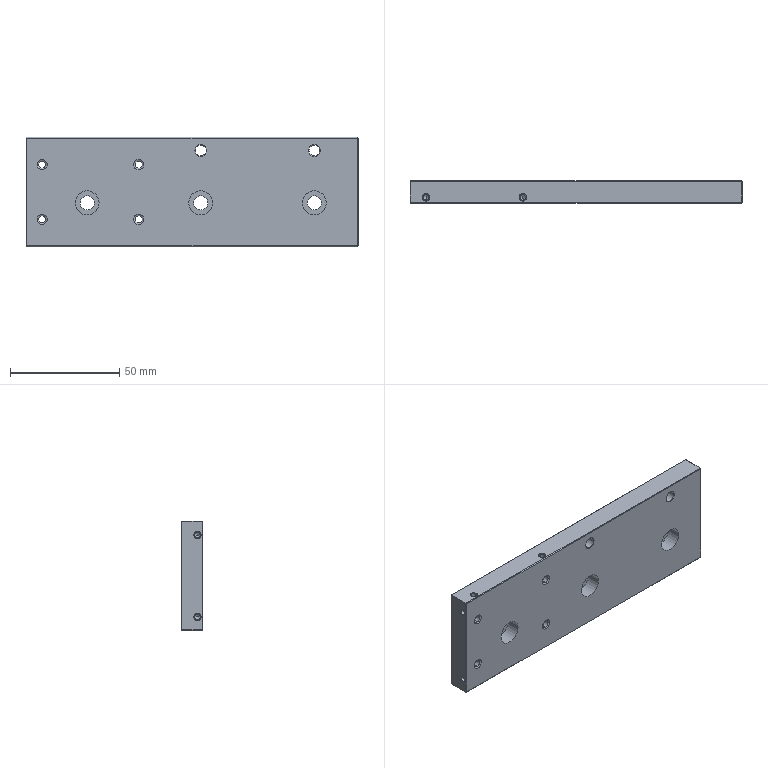Part | NX | 1 solid | 94 faces | box 152 x 10 x 50 mm | volume 72846 mm3 | cylinder 46 | cone 28 | plane 20 | commonest cylinder face diameters 2.5 x22 3.3 x8 6.5 x6 11 x6 5 x4